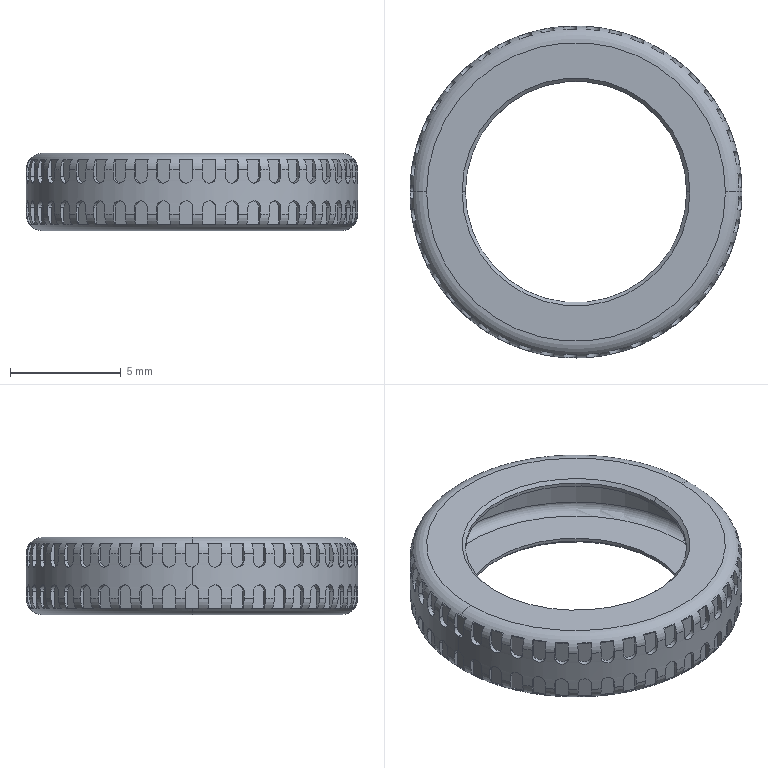Part | SolidWorks | features Chamfer 1, CirPattern 1, Extrusion 1, Fillet 1, ICE 1, Shell 1 | 1 solid | 475 faces | box 15 x 15 x 3.5 mm | volume 81.767 mm3 | plane 364 | cylinder 99 | torus 8 | cone 4 | commonest cylinder face diameters 0.6 x91 10 x4 14.4 x2 15 x2